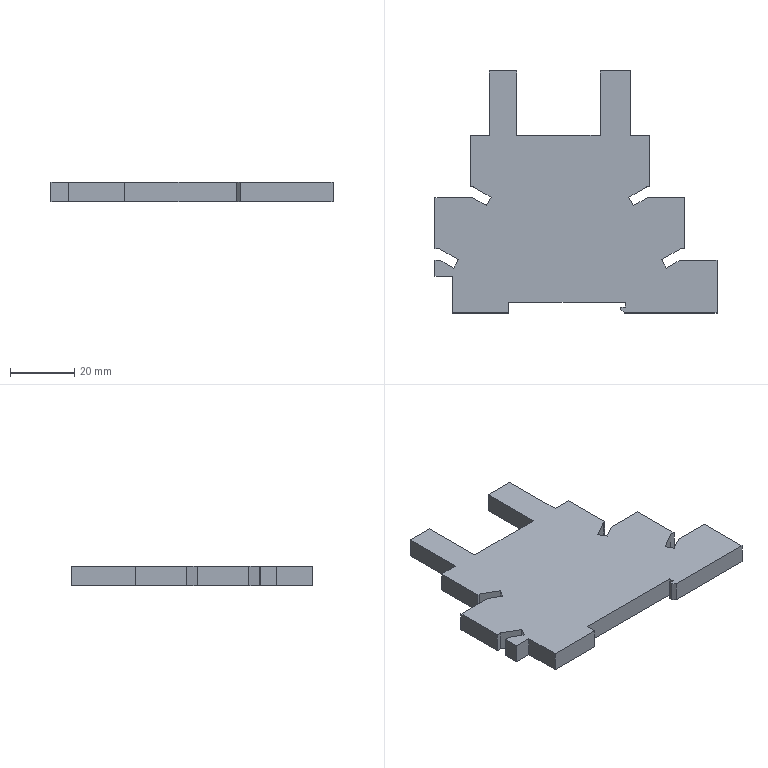Part | STEP file | Ultra-miniature medium-power relay HF41F_24-ZST and socket 41F-1Z-C2-1 | 1 solid | 47 faces | box 88 x 75.5 x 6.1 mm | volume 25363 mm3 | plane 47